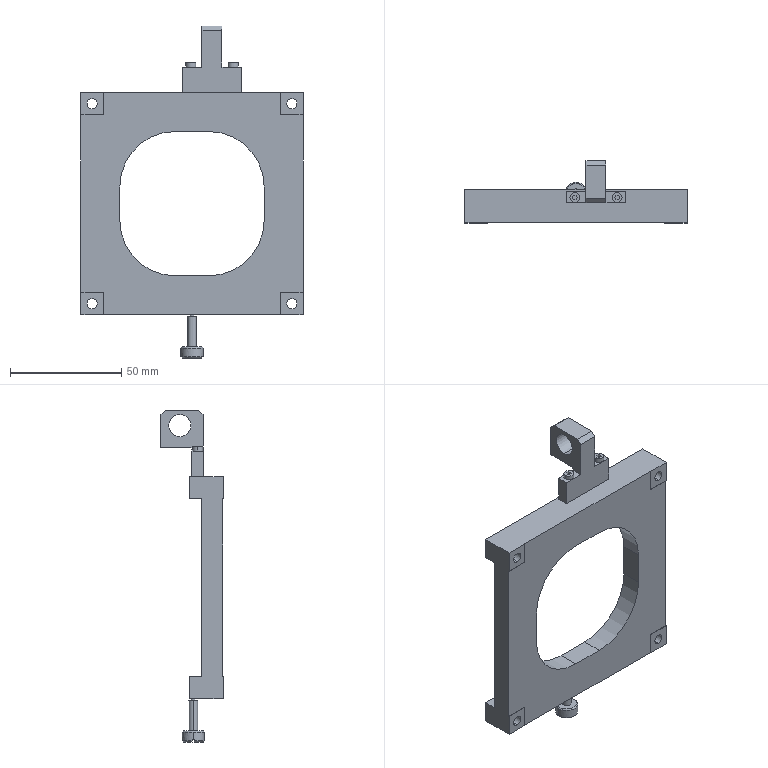Part | SolidWorks | features ICE 9, RevCut 4, Extrusion 1, Revolution 1 | 1 solid | 102 faces | box 100 x 28 x 149.5 mm | volume 72499 mm3 | plane 66 | cylinder 32 | cone 4 | commonest cylinder face diameters 4.5 x12 8 x8 10 x4 50 x4 2 x2 4 x2